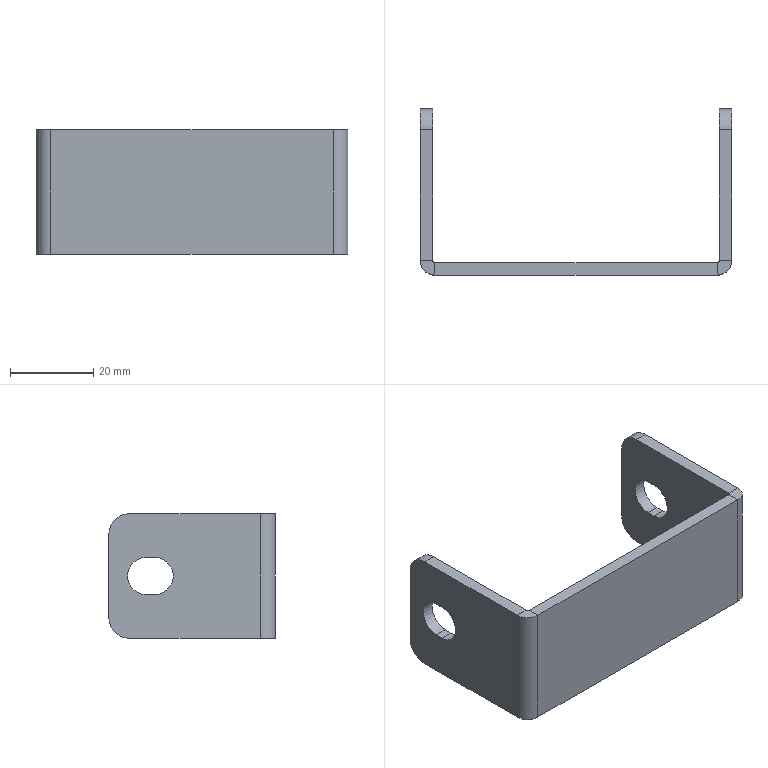Part | STEP file | 7100507 | 1 solid | 34 faces | box 75 x 40 x 30 mm | volume 12701 mm3 | plane 22 | cylinder 12 | commonest cylinder face diameters 9 x4 10 x4 1 x2 7 x2